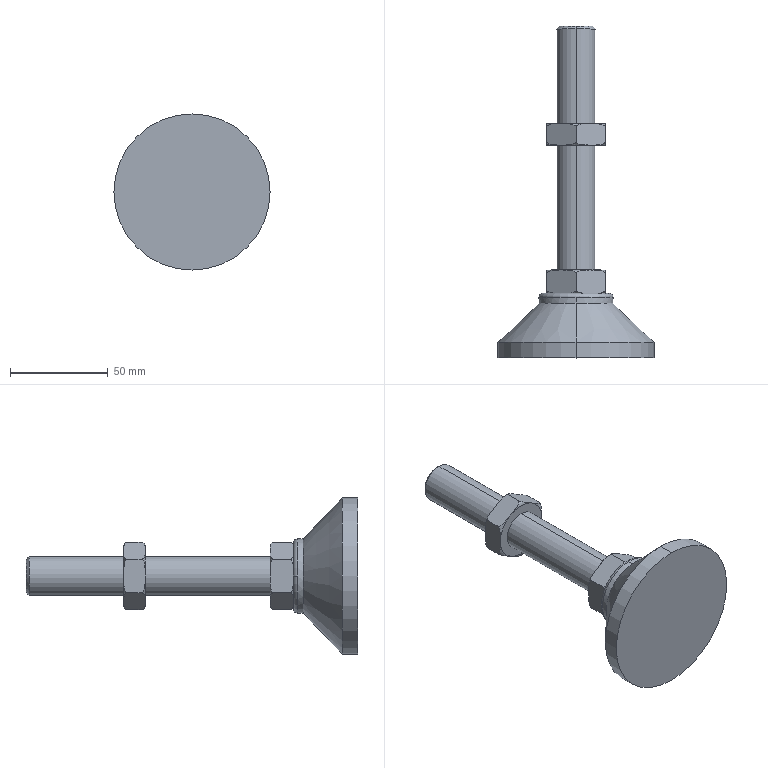Part | SolidWorks | 2 solids | 64 faces | box 80 x 170 x 80 mm | volume 157008 mm3 | torus 30 | plane 18 | cylinder 8 | cone 8 | commonest cylinder face diameters 17.294 x2 20 x2 38 x2 80 x2